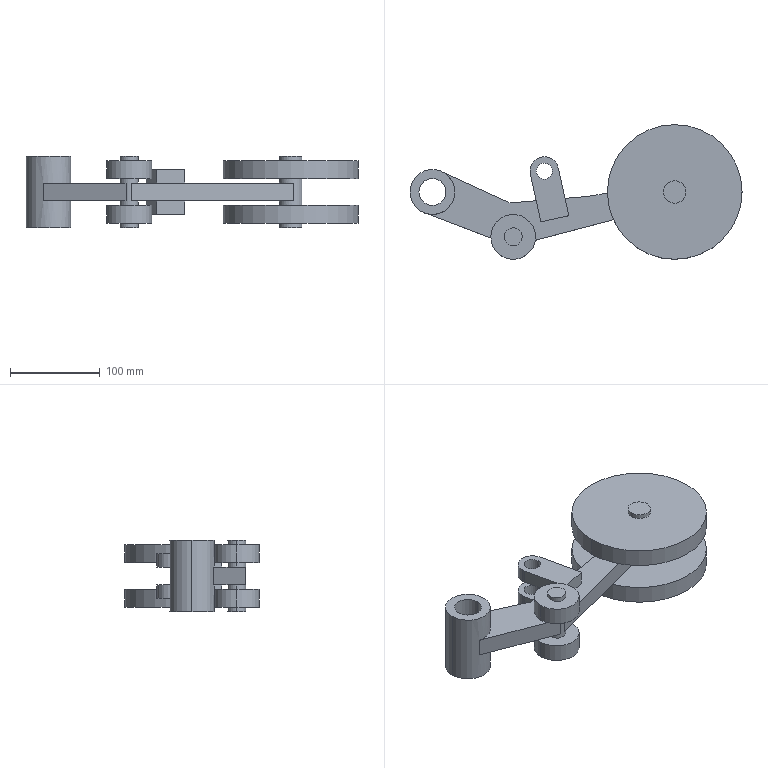Part | SolidWorks | features ICE 4, Extrusion 1, MirrorSolid 1 | 1 solid | 64 faces | box 370 x 150 x 80 mm | volume 1159902 mm3 | cylinder 33 | plane 31 | commonest cylinder face diameters 20 x7 25 x6 50 x6 18 x4 32 x4 150 x4